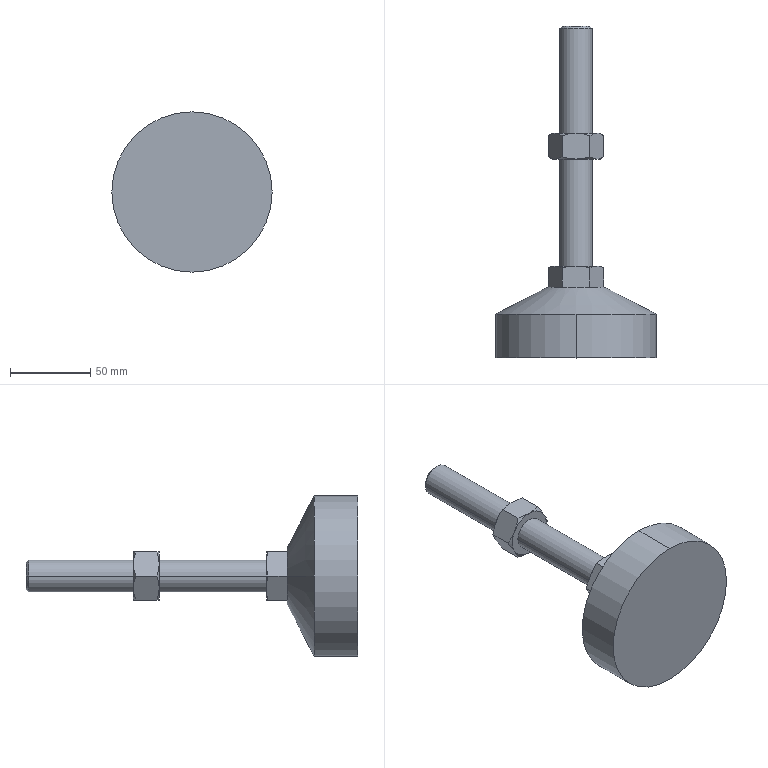Part | STEP file | WAM05-D100-M16-L100 | 2 solids | 53 faces | box 100 x 207 x 100 mm | volume 345017 mm3 | cone 29 | plane 18 | cylinder 6 | commonest cylinder face diameters 17.294 x2 20 x2 100 x2